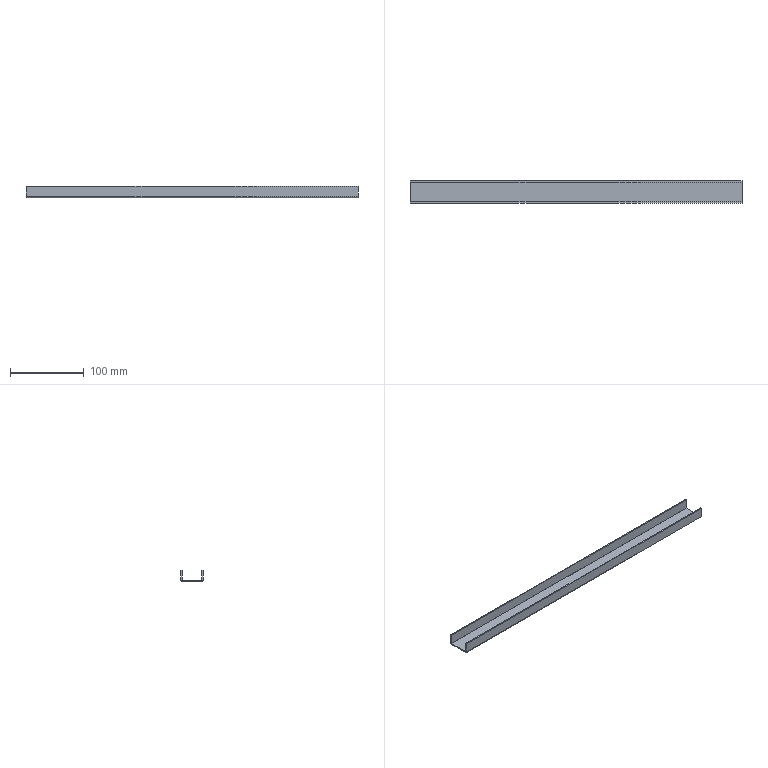Part | SolidWorks | features SplitBody 1 | 1 solid | 22 faces | box 450 x 30 x 15 mm | volume 37982 mm3 | plane 18 | cylinder 4 | commonest cylinder face diameters 0.2 x2 3.2 x2
STEP:
#1=CARTESIAN_POINT('',(-25.,28.4,185.));
#2=VERTEX_POINT('',#1);
#3=CARTESIAN_POINT('',(-25.,28.4,186.5));
#4=VERTEX_POINT('',#3);
#5=CARTESIAN_POINT('',(-25.,28.4,185.));
#6=DIRECTION('',(0.,0.,1.));
#7=VECTOR('',#6,1000.);
#8=LINE('',#5,#7);
#9=EDGE_CURVE('',#2,#4,#8,.T.);
#10=ORIENTED_EDGE('',*,*,#9,.F.);
#11=CARTESIAN_POINT('',(-25.,30.,186.6));
#12=VERTEX_POINT('',#11);
#13=CARTESIAN_POINT('',(-25.,28.4,186.6));
#14=DIRECTION('',(1.,0.,0.));
#15=DIRECTION('',(0.,0.,-1.));
#16=AXIS2_PLACEMENT_3D('',#13,#14,#15);
#17=CIRCLE('',#16,1.6);
#18=EDGE_CURVE('',#2,#12,#17,.T.);
#19=ORIENTED_EDGE('',*,*,#18,.T.);
#20=CARTESIAN_POINT('',(-25.,28.5,186.6));
#21=VERTEX_POINT('',#20);
#22=CARTESIAN_POINT('',(-25.,28.5,186.6));
#23=DIRECTION('',(0.,1.,0.));
#24=VECTOR('',#23,1000.);
#25=LINE('',#22,#24);
#26=EDGE_CURVE('',#21,#12,#25,.T.);
#27=ORIENTED_EDGE('',*,*,#26,.F.);
#28=CARTESIAN_POINT('',(-25.,28.4,186.6));
#29=DIRECTION('',(1.,0.,0.));
#30=DIRECTION('',(0.,0.,1.));
#31=AXIS2_PLACEMENT_3D('',#28,#29,#30);
#32=CIRCLE('',#31,0.1);
#33=EDGE_CURVE('',#4,#21,#32,.T.);
#34=ORIENTED_EDGE('',*,*,#33,.F.);
#35=EDGE_LOOP('',(#10,#19,#27,#34));
#36=FACE_OUTER_BOUND('',#35,.T.);
#37=CARTESIAN_POINT('',(-25.,28.4,185.));
#38=DIRECTION('',(1.,0.,0.));
#39=DIRECTION('',(0.,0.,-1.));
#40=AXIS2_PLACEMENT_3D('',#37,#38,#39);
#41=PLANE('',#40);
#42=ADVANCED_FACE('',(#36),#41,.T.);
#43=CARTESIAN_POINT('',(-25.,1.6,185.));
#44=VERTEX_POINT('',#43);
#45=CARTESIAN_POINT('',(-25.,30.,185.));
#46=DIRECTION('',(0.,1.,0.));
#47=VECTOR('',#46,1000.);
#48=LINE('',#45,#47);
#49=EDGE_CURVE('',#44,#2,#48,.T.);
#50=ORIENTED_EDGE('',*,*,#49,.T.);
#51=ORIENTED_EDGE('',*,*,#9,.T.);
#52=CARTESIAN_POINT('',(-25.,1.6,186.5));
#53=VERTEX_POINT('',#52);
#54=CARTESIAN_POINT('',(-25.,30.,186.5));
#55=DIRECTION('',(0.,1.,0.));
#56=VECTOR('',#55,1000.);
#57=LINE('',#54,#56);
#58=EDGE_CURVE('',#53,#4,#57,.T.);
#59=ORIENTED_EDGE('',*,*,#58,.F.);
#60=CARTESIAN_POINT('',(-25.,1.6,186.5));
#61=DIRECTION('',(0.,0.,-1.));
#62=VECTOR('',#61,1000.);
#63=LINE('',#60,#62);
#64=EDGE_CURVE('',#53,#44,#63,.T.);
#65=ORIENTED_EDGE('',*,*,#64,.T.);
#66=EDGE_LOOP('',(#50,#51,#59,#65));
#67=FACE_OUTER_BOUND('',#66,.T.);
#68=CARTESIAN_POINT('',(-25.,28.5,186.6));
#69=DIRECTION('',(1.,0.,0.));
#70=DIRECTION('',(0.,0.,-1.));
#71=AXIS2_PLACEMENT_3D('',#68,#69,#70);
#72=PLANE('',#71);
#73=ADVANCED_FACE('',(#67),#72,.T.);
#74=CARTESIAN_POINT('',(-25.,0.,186.6));
#75=VERTEX_POINT('',#74);
#76=CARTESIAN_POINT('',(-25.,1.5,186.6));
#77=VERTEX_POINT('',#76);
#78=CARTESIAN_POINT('',(-25.,0.,186.6));
#79=DIRECTION('',(0.,1.,0.));
#80=VECTOR('',#79,1000.);
#81=LINE('',#78,#80);
#82=EDGE_CURVE('',#75,#77,#81,.T.);
#83=ORIENTED_EDGE('',*,*,#82,.F.);
#84=CARTESIAN_POINT('',(-25.,1.6,186.6));
#85=DIRECTION('',(1.,0.,0.));
#86=DIRECTION('',(0.,0.,-1.));
#87=AXIS2_PLACEMENT_3D('',#84,#85,#86);
#88=CIRCLE('',#87,1.6);
#89=EDGE_CURVE('',#75,#44,#88,.T.);
#90=ORIENTED_EDGE('',*,*,#89,.T.);
#91=ORIENTED_EDGE('',*,*,#64,.F.);
#92=CARTESIAN_POINT('',(-25.,1.6,186.6));
#93=DIRECTION('',(1.,0.,0.));
#94=DIRECTION('',(0.,0.,1.));
#95=AXIS2_PLACEMENT_3D('',#92,#93,#94);
#96=CIRCLE('',#95,0.1);
#97=EDGE_CURVE('',#77,#53,#96,.T.);
#98=ORIENTED_EDGE('',*,*,#97,.F.);
#99=EDGE_LOOP('',(#83,#90,#91,#98));
#100=FACE_OUTER_BOUND('',#99,.T.);
#101=CARTESIAN_POINT('',(-25.,0.,186.6));
#102=DIRECTION('',(1.,0.,0.));
#103=DIRECTION('',(0.,0.,-1.));
#104=AXIS2_PLACEMENT_3D('',#101,#102,#103);
#105=PLANE('',#104);
#106=ADVANCED_FACE('',(#100),#105,.T.);
#107=CARTESIAN_POINT('',(-25.,0.,200.));
#108=VERTEX_POINT('',#107);
#109=CARTESIAN_POINT('',(-25.,0.,200.));
#110=DIRECTION('',(0.,0.,-1.));
#111=VECTOR('',#110,1000.);
#112=LINE('',#109,#111);
#113=EDGE_CURVE('',#108,#75,#112,.T.);
#114=ORIENTED_EDGE('',*,*,#113,.T.);
#115=ORIENTED_EDGE('',*,*,#82,.T.);
#116=CARTESIAN_POINT('',(-25.,1.5,200.));
#117=VERTEX_POINT('',#116);
#118=CARTESIAN_POINT('',(-25.,1.5,200.));
#119=DIRECTION('',(0.,0.,-1.));
#120=VECTOR('',#119,1000.);
#121=LINE('',#118,#120);
#122=EDGE_CURVE('',#117,#77,#121,.T.);
#123=ORIENTED_EDGE('',*,*,#122,.F.);
#124=CARTESIAN_POINT('',(-25.,1.5,200.));
#125=DIRECTION('',(0.,-1.,0.));
#126=VECTOR('',#125,1000.);
#127=LINE('',#124,#126);
#128=EDGE_CURVE('',#117,#108,#127,.T.);
#129=ORIENTED_EDGE('',*,*,#128,.T.);
#130=EDGE_LOOP('',(#114,#115,#123,#129));
#131=FACE_OUTER_BOUND('',#130,.T.);
#132=CARTESIAN_POINT('',(-25.,1.6,186.5));
#133=DIRECTION('',(1.,0.,0.));
#134=DIRECTION('',(0.,0.,-1.));
#135=AXIS2_PLACEMENT_3D('',#132,#133,#134);
#136=PLANE('',#135);
#137=ADVANCED_FACE('',(#131),#136,.T.);
#138=CARTESIAN_POINT('',(-475.,28.5,186.6));
#139=VERTEX_POINT('',#138);
#140=CARTESIAN_POINT('',(-475.,28.5,200.));
#141=VERTEX_POINT('',#140);
#142=CARTESIAN_POINT('',(-475.,28.5,185.));
#143=DIRECTION('',(0.,0.,1.));
#144=VECTOR('',#143,1000.);
#145=LINE('',#142,#144);
#146=EDGE_CURVE('',#139,#141,#145,.T.);
#147=ORIENTED_EDGE('',*,*,#146,.F.);
#148=CARTESIAN_POINT('',(-508.541,28.5,186.6));
#149=DIRECTION('',(1.,0.,0.));
#150=VECTOR('',#149,1000.);
#151=LINE('',#148,#150);
#152=EDGE_CURVE('',#139,#21,#151,.T.);
#153=ORIENTED_EDGE('',*,*,#152,.T.);
#154=CARTESIAN_POINT('',(-25.,28.5,200.));
#155=VERTEX_POINT('',#154);
#156=CARTESIAN_POINT('',(-25.,28.5,185.));
#157=DIRECTION('',(0.,0.,1.));
#158=VECTOR('',#157,1000.);
#159=LINE('',#156,#158);
#160=EDGE_CURVE('',#21,#155,#159,.T.);
#161=ORIENTED_EDGE('',*,*,#160,.T.);
#162=CARTESIAN_POINT('',(-508.541,28.5,200.));
#163=DIRECTION('',(1.,0.,0.));
#164=VECTOR('',#163,1000.);
#165=LINE('',#162,#164);
#166=EDGE_CURVE('',#141,#155,#165,.T.);
#167=ORIENTED_EDGE('',*,*,#166,.F.);
#168=EDGE_LOOP('',(#147,#153,#161,#167));
#169=FACE_OUTER_BOUND('',#168,.T.);
#170=CARTESIAN_POINT('',(-508.541,28.5,185.));
#171=DIRECTION('',(0.,1.,0.));
#172=DIRECTION('',(0.,0.,1.));
#173=AXIS2_PLACEMENT_3D('',#170,#171,#172);
#174=PLANE('',#173);
#175=ADVANCED_FACE('',(#169),#174,.F.);
#176=CARTESIAN_POINT('',(-475.,30.,200.));
#177=VERTEX_POINT('',#176);
#178=CARTESIAN_POINT('',(-25.,30.,200.));
#179=VERTEX_POINT('',#178);
#180=CARTESIAN_POINT('',(-508.541,30.,200.));
#181=DIRECTION('',(1.,0.,0.));
#182=VECTOR('',#181,1000.);
#183=LINE('',#180,#182);
#184=EDGE_CURVE('',#177,#179,#183,.T.);
#185=ORIENTED_EDGE('',*,*,#184,.F.);
#186=CARTESIAN_POINT('',(-475.,30.,200.));
#187=DIRECTION('',(0.,-1.,0.));
#188=VECTOR('',#187,1000.);
#189=LINE('',#186,#188);
#190=EDGE_CURVE('',#177,#141,#189,.T.);
#191=ORIENTED_EDGE('',*,*,#190,.T.);
#192=ORIENTED_EDGE('',*,*,#166,.T.);
#193=CARTESIAN_POINT('',(-25.,30.,200.));
#194=DIRECTION('',(0.,-1.,0.));
#195=VECTOR('',#194,1000.);
#196=LINE('',#193,#195);
#197=EDGE_CURVE('',#179,#155,#196,.T.);
#198=ORIENTED_EDGE('',*,*,#197,.F.);
#199=EDGE_LOOP('',(#185,#191,#192,#198));
#200=FACE_OUTER_BOUND('',#199,.T.);
#201=CARTESIAN_POINT('',(-508.541,30.,200.));
#202=DIRECTION('',(0.,0.,1.));
#203=DIRECTION('',(1.,0.,0.));
#204=AXIS2_PLACEMENT_3D('',#201,#202,#203);
#205=PLANE('',#204);
#206=ADVANCED_FACE('',(#200),#205,.T.);
#207=CARTESIAN_POINT('',(-475.,30.,186.6));
#208=VERTEX_POINT('',#207);
#209=CARTESIAN_POINT('',(-508.541,30.,186.6));
#210=DIRECTION('',(1.,0.,0.));
#211=VECTOR('',#210,1000.);
#212=LINE('',#209,#211);
#213=EDGE_CURVE('',#208,#12,#212,.T.);
#214=ORIENTED_EDGE('',*,*,#213,.F.);
#215=CARTESIAN_POINT('',(-475.,30.,185.));
#216=DIRECTION('',(0.,0.,1.));
#217=VECTOR('',#216,1000.);
#218=LINE('',#215,#217);
#219=EDGE_CURVE('',#208,#177,#218,.T.);
#220=ORIENTED_EDGE('',*,*,#219,.T.);
#221=ORIENTED_EDGE('',*,*,#184,.T.);
#222=CARTESIAN_POINT('',(-25.,30.,185.));
#223=DIRECTION('',(0.,0.,1.));
#224=VECTOR('',#223,1000.);
#225=LINE('',#222,#224);
#226=EDGE_CURVE('',#12,#179,#225,.T.);
#227=ORIENTED_EDGE('',*,*,#226,.F.);
#228=EDGE_LOOP('',(#214,#220,#221,#227));
#229=FACE_OUTER_BOUND('',#228,.T.);
#230=CARTESIAN_POINT('',(-508.541,30.,185.));
#231=DIRECTION('',(0.,1.,0.));
#232=DIRECTION('',(0.,0.,1.));
#233=AXIS2_PLACEMENT_3D('',#230,#231,#232);
#234=PLANE('',#233);
#235=ADVANCED_FACE('',(#229),#234,.T.);
#236=CARTESIAN_POINT('',(-475.,28.4,185.));
#237=VERTEX_POINT('',#236);
#238=CARTESIAN_POINT('',(-508.541,28.4,185.));
#239=DIRECTION('',(1.,0.,0.));
#240=VECTOR('',#239,1000.);
#241=LINE('',#238,#240);
#242=EDGE_CURVE('',#237,#2,#241,.T.);
#243=ORIENTED_EDGE('',*,*,#242,.F.);
#244=CARTESIAN_POINT('',(-475.,28.4,186.6));
#245=DIRECTION('',(-1.,0.,0.));
#246=DIRECTION('',(0.,0.,-1.));
#247=AXIS2_PLACEMENT_3D('',#244,#245,#246);
#248=CIRCLE('',#247,1.6);
#249=EDGE_CURVE('',#208,#237,#248,.T.);
#250=ORIENTED_EDGE('',*,*,#249,.F.);
#251=ORIENTED_EDGE('',*,*,#213,.T.);
#252=ORIENTED_EDGE('',*,*,#18,.F.);
#253=EDGE_LOOP('',(#243,#250,#251,#252));
#254=FACE_OUTER_BOUND('',#253,.T.);
#255=CARTESIAN_POINT('',(-508.541,28.4,186.6));
#256=DIRECTION('',(1.,0.,0.));
#257=DIRECTION('',(0.,0.,-1.));
#258=AXIS2_PLACEMENT_3D('',#255,#256,#257);
#259=CYLINDRICAL_SURFACE('',#258,1.6);
#260=ADVANCED_FACE('',(#254),#259,.T.);
#261=CARTESIAN_POINT('',(-475.,1.6,185.));
#262=VERTEX_POINT('',#261);
#263=CARTESIAN_POINT('',(-508.541,1.6,185.));
#264=DIRECTION('',(1.,0.,0.));
#265=VECTOR('',#264,1000.);
#266=LINE('',#263,#265);
#267=EDGE_CURVE('',#262,#44,#266,.T.);
#268=ORIENTED_EDGE('',*,*,#267,.F.);
#269=CARTESIAN_POINT('',(-475.,30.,185.));
#270=DIRECTION('',(0.,1.,0.));
#271=VECTOR('',#270,1000.);
#272=LINE('',#269,#271);
#273=EDGE_CURVE('',#262,#237,#272,.T.);
#274=ORIENTED_EDGE('',*,*,#273,.T.);
#275=ORIENTED_EDGE('',*,*,#242,.T.);
#276=ORIENTED_EDGE('',*,*,#49,.F.);
#277=EDGE_LOOP('',(#268,#274,#275,#276));
#278=FACE_OUTER_BOUND('',#277,.T.);
#279=CARTESIAN_POINT('',(-508.541,30.,185.));
#280=DIRECTION('',(0.,0.,-1.));
#281=DIRECTION('',(-1.,0.,0.));
#282=AXIS2_PLACEMENT_3D('',#279,#280,#281);
#283=PLANE('',#282);
#284=ADVANCED_FACE('',(#278),#283,.T.);
#285=CARTESIAN_POINT('',(-475.,0.,186.6));
#286=VERTEX_POINT('',#285);
#287=CARTESIAN_POINT('',(-508.541,0.,186.6));
#288=DIRECTION('',(1.,0.,0.));
#289=VECTOR('',#288,1000.);
#290=LINE('',#287,#289);
#291=EDGE_CURVE('',#286,#75,#290,.T.);
#292=ORIENTED_EDGE('',*,*,#291,.F.);
#293=CARTESIAN_POINT('',(-475.,1.6,186.6));
#294=DIRECTION('',(-1.,0.,0.));
#295=DIRECTION('',(0.,0.,-1.));
#296=AXIS2_PLACEMENT_3D('',#293,#294,#295);
#297=CIRCLE('',#296,1.6);
#298=EDGE_CURVE('',#262,#286,#297,.T.);
#299=ORIENTED_EDGE('',*,*,#298,.F.);
#300=ORIENTED_EDGE('',*,*,#267,.T.);
#301=ORIENTED_EDGE('',*,*,#89,.F.);
#302=EDGE_LOOP('',(#292,#299,#300,#301));
#303=FACE_OUTER_BOUND('',#302,.T.);
#304=CARTESIAN_POINT('',(-508.541,1.6,186.6));
#305=DIRECTION('',(1.,0.,0.));
#306=DIRECTION('',(0.,0.,-1.));
#307=AXIS2_PLACEMENT_3D('',#304,#305,#306);
#308=CYLINDRICAL_SURFACE('',#307,1.6);
#309=ADVANCED_FACE('',(#303),#308,.T.);
#310=CARTESIAN_POINT('',(-475.,0.,200.));
#311=VERTEX_POINT('',#310);
#312=CARTESIAN_POINT('',(-508.541,0.,200.));
#313=DIRECTION('',(1.,0.,0.));
#314=VECTOR('',#313,1000.);
#315=LINE('',#312,#314);
#316=EDGE_CURVE('',#311,#108,#315,.T.);
#317=ORIENTED_EDGE('',*,*,#316,.F.);
#318=CARTESIAN_POINT('',(-475.,0.,200.));
#319=DIRECTION('',(0.,0.,-1.));
#320=VECTOR('',#319,1000.);
#321=LINE('',#318,#320);
#322=EDGE_CURVE('',#311,#286,#321,.T.);
#323=ORIENTED_EDGE('',*,*,#322,.T.);
#324=ORIENTED_EDGE('',*,*,#291,.T.);
#325=ORIENTED_EDGE('',*,*,#113,.F.);
#326=EDGE_LOOP('',(#317,#323,#324,#325));
#327=FACE_OUTER_BOUND('',#326,.T.);
#328=CARTESIAN_POINT('',(-508.541,0.,200.));
#329=DIRECTION('',(0.,-1.,0.));
#330=DIRECTION('',(0.,0.,-1.));
#331=AXIS2_PLACEMENT_3D('',#328,#329,#330);
#332=PLANE('',#331);
#333=ADVANCED_FACE('',(#327),#332,.T.);
#334=CARTESIAN_POINT('',(-475.,1.5,200.));
#335=VERTEX_POINT('',#334);
#336=CARTESIAN_POINT('',(-508.541,1.5,200.));
#337=DIRECTION('',(1.,0.,0.));
#338=VECTOR('',#337,1000.);
#339=LINE('',#336,#338);
#340=EDGE_CURVE('',#335,#117,#339,.T.);
#341=ORIENTED_EDGE('',*,*,#340,.F.);
#342=CARTESIAN_POINT('',(-475.,1.5,200.));
#343=DIRECTION('',(0.,-1.,0.));
#344=VECTOR('',#343,1000.);
#345=LINE('',#342,#344);
#346=EDGE_CURVE('',#335,#311,#345,.T.);
#347=ORIENTED_EDGE('',*,*,#346,.T.);
#348=ORIENTED_EDGE('',*,*,#316,.T.);
#349=ORIENTED_EDGE('',*,*,#128,.F.);
#350=EDGE_LOOP('',(#341,#347,#348,#349));
#351=FACE_OUTER_BOUND('',#350,.T.);
#352=CARTESIAN_POINT('',(-508.541,1.5,200.));
#353=DIRECTION('',(0.,0.,1.));
#354=DIRECTION('',(1.,0.,0.));
#355=AXIS2_PLACEMENT_3D('',#352,#353,#354);
#356=PLANE('',#355);
#357=ADVANCED_FACE('',(#351),#356,.T.);
#358=CARTESIAN_POINT('',(-475.,1.5,186.6));
#359=VERTEX_POINT('',#358);
#360=CARTESIAN_POINT('',(-475.,1.5,200.));
#361=DIRECTION('',(0.,0.,-1.));
#362=VECTOR('',#361,1000.);
#363=LINE('',#360,#362);
#364=EDGE_CURVE('',#335,#359,#363,.T.);
#365=ORIENTED_EDGE('',*,*,#364,.F.);
#366=ORIENTED_EDGE('',*,*,#340,.T.);
#367=ORIENTED_EDGE('',*,*,#122,.T.);
#368=CARTESIAN_POINT('',(-508.541,1.5,186.6));
#369=DIRECTION('',(1.,0.,0.));
#370=VECTOR('',#369,1000.);
#371=LINE('',#368,#370);
#372=EDGE_CURVE('',#359,#77,#371,.T.);
#373=ORIENTED_EDGE('',*,*,#372,.F.);
#374=EDGE_LOOP('',(#365,#366,#367,#373));
#375=FACE_OUTER_BOUND('',#374,.T.);
#376=CARTESIAN_POINT('',(-508.541,1.5,200.));
#377=DIRECTION('',(0.,-1.,0.));
#378=DIRECTION('',(0.,0.,-1.));
#379=AXIS2_PLACEMENT_3D('',#376,#377,#378);
#380=PLANE('',#379);
#381=ADVANCED_FACE('',(#375),#380,.F.);
#382=CARTESIAN_POINT('',(-475.,1.6,186.5));
#383=VERTEX_POINT('',#382);
#384=CARTESIAN_POINT('',(-475.,1.6,186.6));
#385=DIRECTION('',(1.,0.,0.));
#386=DIRECTION('',(0.,0.,1.));
#387=AXIS2_PLACEMENT_3D('',#384,#385,#386);
#388=CIRCLE('',#387,0.1);
#389=EDGE_CURVE('',#359,#383,#388,.T.);
#390=ORIENTED_EDGE('',*,*,#389,.F.);
#391=ORIENTED_EDGE('',*,*,#372,.T.);
#392=ORIENTED_EDGE('',*,*,#97,.T.);
#393=CARTESIAN_POINT('',(-508.541,1.6,186.5));
#394=DIRECTION('',(1.,0.,0.));
#395=VECTOR('',#394,1000.);
#396=LINE('',#393,#395);
#397=EDGE_CURVE('',#383,#53,#396,.T.);
#398=ORIENTED_EDGE('',*,*,#397,.F.);
#399=EDGE_LOOP('',(#390,#391,#392,#398));
#400=FACE_OUTER_BOUND('',#399,.T.);
#401=CARTESIAN_POINT('',(-508.541,1.6,186.6));
#402=DIRECTION('',(1.,0.,0.));
#403=DIRECTION('',(0.,0.,-1.));
#404=AXIS2_PLACEMENT_3D('',#401,#402,#403);
#405=CYLINDRICAL_SURFACE('',#404,0.1);
#406=ADVANCED_FACE('',(#400),#405,.F.);
#407=CARTESIAN_POINT('',(-475.,28.4,186.5));
#408=VERTEX_POINT('',#407);
#409=CARTESIAN_POINT('',(-475.,30.,186.5));
#410=DIRECTION('',(0.,1.,0.));
#411=VECTOR('',#410,1000.);
#412=LINE('',#409,#411);
#413=EDGE_CURVE('',#383,#408,#412,.T.);
#414=ORIENTED_EDGE('',*,*,#413,.F.);
#415=ORIENTED_EDGE('',*,*,#397,.T.);
#416=ORIENTED_EDGE('',*,*,#58,.T.);
#417=CARTESIAN_POINT('',(-508.541,28.4,186.5));
#418=DIRECTION('',(1.,0.,0.));
#419=VECTOR('',#418,1000.);
#420=LINE('',#417,#419);
#421=EDGE_CURVE('',#408,#4,#420,.T.);
#422=ORIENTED_EDGE('',*,*,#421,.F.);
#423=EDGE_LOOP('',(#414,#415,#416,#422));
#424=FACE_OUTER_BOUND('',#423,.T.);
#425=CARTESIAN_POINT('',(-508.541,30.,186.5));
#426=DIRECTION('',(0.,0.,-1.));
#427=DIRECTION('',(-1.,0.,0.));
#428=AXIS2_PLACEMENT_3D('',#425,#426,#427);
#429=PLANE('',#428);
#430=ADVANCED_FACE('',(#424),#429,.F.);
#431=CARTESIAN_POINT('',(-475.,28.4,186.6));
#432=DIRECTION('',(1.,0.,0.));
#433=DIRECTION('',(0.,0.,1.));
#434=AXIS2_PLACEMENT_3D('',#431,#432,#433);
#435=CIRCLE('',#434,0.1);
#436=EDGE_CURVE('',#408,#139,#435,.T.);
#437=ORIENTED_EDGE('',*,*,#436,.F.);
#438=ORIENTED_EDGE('',*,*,#421,.T.);
#439=ORIENTED_EDGE('',*,*,#33,.T.);
#440=ORIENTED_EDGE('',*,*,#152,.F.);
#441=EDGE_LOOP('',(#437,#438,#439,#440));
#442=FACE_OUTER_BOUND('',#441,.T.);
#443=CARTESIAN_POINT('',(-508.541,28.4,186.6));
#444=DIRECTION('',(1.,0.,0.));
#445=DIRECTION('',(0.,0.,-1.));
#446=AXIS2_PLACEMENT_3D('',#443,#444,#445);
#447=CYLINDRICAL_SURFACE('',#446,0.1);
#448=ADVANCED_FACE('',(#442),#447,.F.);
#449=ORIENTED_EDGE('',*,*,#160,.F.);
#450=ORIENTED_EDGE('',*,*,#26,.T.);
#451=ORIENTED_EDGE('',*,*,#226,.T.);
#452=ORIENTED_EDGE('',*,*,#197,.T.);
#453=EDGE_LOOP('',(#449,#450,#451,#452));
#454=FACE_OUTER_BOUND('',#453,.T.);
#455=CARTESIAN_POINT('',(-25.,28.4,186.6));
#456=DIRECTION('',(1.,0.,0.));
#457=DIRECTION('',(0.,0.,-1.));
#458=AXIS2_PLACEMENT_3D('',#455,#456,#457);
#459=PLANE('',#458);
#460=ADVANCED_FACE('',(#454),#459,.T.);
#461=ORIENTED_EDGE('',*,*,#413,.T.);
#462=CARTESIAN_POINT('',(-475.,28.4,186.5));
#463=DIRECTION('',(0.,0.,-1.));
#464=VECTOR('',#463,1000.);
#465=LINE('',#462,#464);
#466=EDGE_CURVE('',#408,#237,#465,.T.);
#467=ORIENTED_EDGE('',*,*,#466,.T.);
#468=ORIENTED_EDGE('',*,*,#273,.F.);
#469=CARTESIAN_POINT('',(-475.,1.6,186.5));
#470=DIRECTION('',(0.,0.,-1.));
#471=VECTOR('',#470,1000.);
#472=LINE('',#469,#471);
#473=EDGE_CURVE('',#383,#262,#472,.T.);
#474=ORIENTED_EDGE('',*,*,#473,.F.);
#475=EDGE_LOOP('',(#461,#467,#468,#474));
#476=FACE_OUTER_BOUND('',#475,.T.);
#477=CARTESIAN_POINT('',(-475.,30.,186.5));
#478=DIRECTION('',(-1.,0.,0.));
#479=DIRECTION('',(0.,1.,0.));
#480=AXIS2_PLACEMENT_3D('',#477,#478,#479);
#481=PLANE('',#480);
#482=ADVANCED_FACE('',(#476),#481,.T.);
#483=ORIENTED_EDGE('',*,*,#364,.T.);
#484=CARTESIAN_POINT('',(-475.,1.5,186.6));
#485=DIRECTION('',(0.,-1.,0.));
#486=VECTOR('',#485,1000.);
#487=LINE('',#484,#486);
#488=EDGE_CURVE('',#359,#286,#487,.T.);
#489=ORIENTED_EDGE('',*,*,#488,.T.);
#490=ORIENTED_EDGE('',*,*,#322,.F.);
#491=ORIENTED_EDGE('',*,*,#346,.F.);
#492=EDGE_LOOP('',(#483,#489,#490,#491));
#493=FACE_OUTER_BOUND('',#492,.T.);
#494=CARTESIAN_POINT('',(-475.,1.5,200.));
#495=DIRECTION('',(-1.,0.,0.));
#496=DIRECTION('',(0.,0.,-1.));
#497=AXIS2_PLACEMENT_3D('',#494,#495,#496);
#498=PLANE('',#497);
#499=ADVANCED_FACE('',(#493),#498,.T.);
#500=ORIENTED_EDGE('',*,*,#298,.T.);
#501=ORIENTED_EDGE('',*,*,#488,.F.);
#502=ORIENTED_EDGE('',*,*,#389,.T.);
#503=ORIENTED_EDGE('',*,*,#473,.T.);
#504=EDGE_LOOP('',(#500,#501,#502,#503));
#505=FACE_OUTER_BOUND('',#504,.T.);
#506=CARTESIAN_POINT('',(-475.,1.6,186.6));
#507=DIRECTION('',(1.,0.,0.));
#508=DIRECTION('',(0.,0.,-1.));
#509=AXIS2_PLACEMENT_3D('',#506,#507,#508);
#510=PLANE('',#509);
#511=ADVANCED_FACE('',(#505),#510,.F.);
#512=ORIENTED_EDGE('',*,*,#190,.F.);
#513=ORIENTED_EDGE('',*,*,#219,.F.);
#514=CARTESIAN_POINT('',(-475.,30.,186.6));
#515=DIRECTION('',(0.,-1.,0.));
#516=VECTOR('',#515,1000.);
#517=LINE('',#514,#516);
#518=EDGE_CURVE('',#208,#139,#517,.T.);
#519=ORIENTED_EDGE('',*,*,#518,.T.);
#520=ORIENTED_EDGE('',*,*,#146,.T.);
#521=EDGE_LOOP('',(#512,#513,#519,#520));
#522=FACE_OUTER_BOUND('',#521,.T.);
#523=CARTESIAN_POINT('',(-475.,30.,185.));
#524=DIRECTION('',(-1.,0.,0.));
#525=DIRECTION('',(0.,0.,1.));
#526=AXIS2_PLACEMENT_3D('',#523,#524,#525);
#527=PLANE('',#526);
#528=ADVANCED_FACE('',(#522),#527,.T.);
#529=ORIENTED_EDGE('',*,*,#249,.T.);
#530=ORIENTED_EDGE('',*,*,#466,.F.);
#531=ORIENTED_EDGE('',*,*,#436,.T.);
#532=ORIENTED_EDGE('',*,*,#518,.F.);
#533=EDGE_LOOP('',(#529,#530,#531,#532));
#534=FACE_OUTER_BOUND('',#533,.T.);
#535=CARTESIAN_POINT('',(-475.,28.4,186.6));
#536=DIRECTION('',(1.,0.,0.));
#537=DIRECTION('',(0.,0.,-1.));
#538=AXIS2_PLACEMENT_3D('',#535,#536,#537);
#539=PLANE('',#538);
#540=ADVANCED_FACE('',(#534),#539,.F.);
#541=CLOSED_SHELL('',(#42,#73,#106,#137,#175,#206,#235,#260,#284,#309,#333,#357,#381,#406,#430,#448,#460,#482,#499,#511,#528,#540));
#542=MANIFOLD_SOLID_BREP('',#541);
#543=CARTESIAN_POINT('',(0.,0.,0.));
#544=DIRECTION('',(0.,0.,1.));
#545=DIRECTION('',(1.,0.,0.));
#546=AXIS2_PLACEMENT_3D('',#543,#544,#545);
#547=(LENGTH_UNIT()NAMED_UNIT(*)SI_UNIT(.MILLI.,.METRE.));
#548=UNCERTAINTY_MEASURE_WITH_UNIT(LENGTH_MEASURE(0.00001),#547,'','');
#549=(NAMED_UNIT(*)PLANE_ANGLE_UNIT()SI_UNIT($,.RADIAN.));
#550=(NAMED_UNIT(*)SI_UNIT($,.STERADIAN.)SOLID_ANGLE_UNIT());
#551=(GEOMETRIC_REPRESENTATION_CONTEXT(3)GLOBAL_UNCERTAINTY_ASSIGNED_CONTEXT((#548))GLOBAL_UNIT_ASSIGNED_CONTEXT((#547,#549,#550))REPRESENTATION_CONTEXT('',''));
#552=ADVANCED_BREP_SHAPE_REPRESENTATION('',(#542,#546),#551);